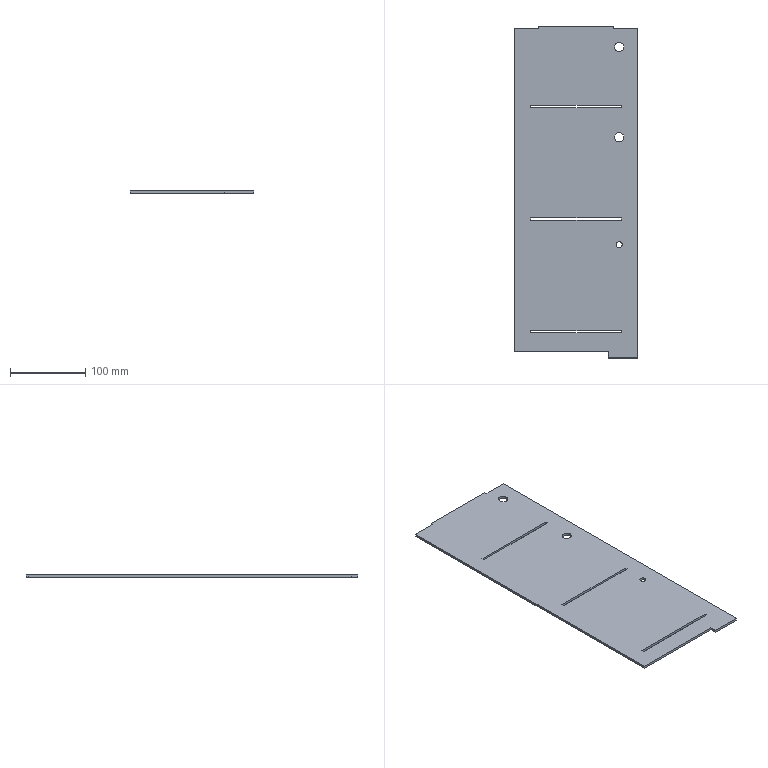Part | SolidWorks | features FlatPattern 1, SMBaseFlange 1, SheetMetal 1 | 1 solid | 30 faces | box 165 x 442 x 3.2 mm | volume 224791 mm3 | plane 24 | cylinder 6 | commonest cylinder face diameters 12.5 x4 8 x2
STEP:
#1=CARTESIAN_POINT('',(-21.25,194.5,3.2));
#2=VERTEX_POINT('',#1);
#3=CARTESIAN_POINT('',(-8.75,194.5,3.2));
#4=VERTEX_POINT('',#3);
#5=CARTESIAN_POINT('',(-15.,194.5,3.2));
#6=DIRECTION('',(0.,0.,1.));
#7=DIRECTION('',(1.,0.,0.));
#8=AXIS2_PLACEMENT_3D('',#5,#6,#7);
#9=CIRCLE('',#8,6.25);
#10=EDGE_CURVE('',#2,#4,#9,.T.);
#11=ORIENTED_EDGE('',*,*,#10,.T.);
#12=CARTESIAN_POINT('',(-8.75,194.5,0.));
#13=VERTEX_POINT('',#12);
#14=CARTESIAN_POINT('',(-8.75,194.5,3.2));
#15=DIRECTION('',(0.,0.,-1.));
#16=VECTOR('',#15,1000.);
#17=LINE('',#14,#16);
#18=EDGE_CURVE('',#4,#13,#17,.T.);
#19=ORIENTED_EDGE('',*,*,#18,.T.);
#20=CARTESIAN_POINT('',(-21.25,194.5,0.));
#21=VERTEX_POINT('',#20);
#22=CARTESIAN_POINT('',(-15.,194.5,0.));
#23=DIRECTION('',(0.,0.,1.));
#24=DIRECTION('',(1.,0.,0.));
#25=AXIS2_PLACEMENT_3D('',#22,#23,#24);
#26=CIRCLE('',#25,6.25);
#27=EDGE_CURVE('',#21,#13,#26,.T.);
#28=ORIENTED_EDGE('',*,*,#27,.F.);
#29=CARTESIAN_POINT('',(-21.25,194.5,3.2));
#30=DIRECTION('',(0.,0.,-1.));
#31=VECTOR('',#30,1000.);
#32=LINE('',#29,#31);
#33=EDGE_CURVE('',#2,#21,#32,.T.);
#34=ORIENTED_EDGE('',*,*,#33,.F.);
#35=EDGE_LOOP('',(#11,#19,#28,#34));
#36=FACE_OUTER_BOUND('',#35,.T.);
#37=CARTESIAN_POINT('',(-15.,194.5,3.2));
#38=DIRECTION('',(0.,0.,-1.));
#39=DIRECTION('',(-1.,0.,0.));
#40=AXIS2_PLACEMENT_3D('',#37,#38,#39);
#41=CYLINDRICAL_SURFACE('',#40,6.25);
#42=ADVANCED_FACE('',(#36),#41,.F.);
#43=CARTESIAN_POINT('',(-21.25,74.5,3.2));
#44=VERTEX_POINT('',#43);
#45=CARTESIAN_POINT('',(-8.75,74.5,3.2));
#46=VERTEX_POINT('',#45);
#47=CARTESIAN_POINT('',(-15.,74.5,3.2));
#48=DIRECTION('',(0.,0.,1.));
#49=DIRECTION('',(1.,0.,0.));
#50=AXIS2_PLACEMENT_3D('',#47,#48,#49);
#51=CIRCLE('',#50,6.25);
#52=EDGE_CURVE('',#44,#46,#51,.T.);
#53=ORIENTED_EDGE('',*,*,#52,.T.);
#54=CARTESIAN_POINT('',(-8.75,74.5,0.));
#55=VERTEX_POINT('',#54);
#56=CARTESIAN_POINT('',(-8.75,74.5,3.2));
#57=DIRECTION('',(0.,0.,-1.));
#58=VECTOR('',#57,1000.);
#59=LINE('',#56,#58);
#60=EDGE_CURVE('',#46,#55,#59,.T.);
#61=ORIENTED_EDGE('',*,*,#60,.T.);
#62=CARTESIAN_POINT('',(-21.25,74.5,0.));
#63=VERTEX_POINT('',#62);
#64=CARTESIAN_POINT('',(-15.,74.5,0.));
#65=DIRECTION('',(0.,0.,1.));
#66=DIRECTION('',(1.,0.,0.));
#67=AXIS2_PLACEMENT_3D('',#64,#65,#66);
#68=CIRCLE('',#67,6.25);
#69=EDGE_CURVE('',#63,#55,#68,.T.);
#70=ORIENTED_EDGE('',*,*,#69,.F.);
#71=CARTESIAN_POINT('',(-21.25,74.5,3.2));
#72=DIRECTION('',(0.,0.,-1.));
#73=VECTOR('',#72,1000.);
#74=LINE('',#71,#73);
#75=EDGE_CURVE('',#44,#63,#74,.T.);
#76=ORIENTED_EDGE('',*,*,#75,.F.);
#77=EDGE_LOOP('',(#53,#61,#70,#76));
#78=FACE_OUTER_BOUND('',#77,.T.);
#79=CARTESIAN_POINT('',(-15.,74.5,3.2));
#80=DIRECTION('',(0.,0.,-1.));
#81=DIRECTION('',(-1.,0.,0.));
#82=AXIS2_PLACEMENT_3D('',#79,#80,#81);
#83=CYLINDRICAL_SURFACE('',#82,6.25);
#84=ADVANCED_FACE('',(#78),#83,.F.);
#85=CARTESIAN_POINT('',(-19.,-68.5,3.2));
#86=VERTEX_POINT('',#85);
#87=CARTESIAN_POINT('',(-11.,-68.5,3.2));
#88=VERTEX_POINT('',#87);
#89=CARTESIAN_POINT('',(-15.,-68.5,3.2));
#90=DIRECTION('',(0.,0.,1.));
#91=DIRECTION('',(1.,0.,0.));
#92=AXIS2_PLACEMENT_3D('',#89,#90,#91);
#93=CIRCLE('',#92,4.);
#94=EDGE_CURVE('',#86,#88,#93,.T.);
#95=ORIENTED_EDGE('',*,*,#94,.T.);
#96=CARTESIAN_POINT('',(-11.,-68.5,0.));
#97=VERTEX_POINT('',#96);
#98=CARTESIAN_POINT('',(-11.,-68.5,3.2));
#99=DIRECTION('',(0.,0.,-1.));
#100=VECTOR('',#99,1000.);
#101=LINE('',#98,#100);
#102=EDGE_CURVE('',#88,#97,#101,.T.);
#103=ORIENTED_EDGE('',*,*,#102,.T.);
#104=CARTESIAN_POINT('',(-19.,-68.5,0.));
#105=VERTEX_POINT('',#104);
#106=CARTESIAN_POINT('',(-15.,-68.5,0.));
#107=DIRECTION('',(0.,0.,1.));
#108=DIRECTION('',(1.,0.,0.));
#109=AXIS2_PLACEMENT_3D('',#106,#107,#108);
#110=CIRCLE('',#109,4.);
#111=EDGE_CURVE('',#105,#97,#110,.T.);
#112=ORIENTED_EDGE('',*,*,#111,.F.);
#113=CARTESIAN_POINT('',(-19.,-68.5,3.2));
#114=DIRECTION('',(0.,0.,-1.));
#115=VECTOR('',#114,1000.);
#116=LINE('',#113,#115);
#117=EDGE_CURVE('',#86,#105,#116,.T.);
#118=ORIENTED_EDGE('',*,*,#117,.F.);
#119=EDGE_LOOP('',(#95,#103,#112,#118));
#120=FACE_OUTER_BOUND('',#119,.T.);
#121=CARTESIAN_POINT('',(-15.,-68.5,3.2));
#122=DIRECTION('',(0.,0.,-1.));
#123=DIRECTION('',(-1.,0.,0.));
#124=AXIS2_PLACEMENT_3D('',#121,#122,#123);
#125=CYLINDRICAL_SURFACE('',#124,4.);
#126=ADVANCED_FACE('',(#120),#125,.F.);
#127=ORIENTED_EDGE('',*,*,#52,.F.);
#128=CARTESIAN_POINT('',(-15.,74.5,3.2));
#129=DIRECTION('',(0.,0.,1.));
#130=DIRECTION('',(1.,0.,0.));
#131=AXIS2_PLACEMENT_3D('',#128,#129,#130);
#132=CIRCLE('',#131,6.25);
#133=EDGE_CURVE('',#46,#44,#132,.T.);
#134=ORIENTED_EDGE('',*,*,#133,.F.);
#135=EDGE_LOOP('',(#127,#134));
#136=FACE_BOUND('',#135,.T.);
#137=CARTESIAN_POINT('',(-122.5,219.5,3.2));
#138=VERTEX_POINT('',#137);
#139=CARTESIAN_POINT('',(-155.,219.5,3.2));
#140=VERTEX_POINT('',#139);
#141=CARTESIAN_POINT('',(-122.5,219.5,3.2));
#142=DIRECTION('',(-1.,0.,0.));
#143=VECTOR('',#142,1000.);
#144=LINE('',#141,#143);
#145=EDGE_CURVE('',#138,#140,#144,.T.);
#146=ORIENTED_EDGE('',*,*,#145,.T.);
#147=CARTESIAN_POINT('',(-155.,-211.2,3.2));
#148=VERTEX_POINT('',#147);
#149=CARTESIAN_POINT('',(-155.,219.5,3.2));
#150=DIRECTION('',(0.,-1.,0.));
#151=VECTOR('',#150,1000.);
#152=LINE('',#149,#151);
#153=EDGE_CURVE('',#140,#148,#152,.T.);
#154=ORIENTED_EDGE('',*,*,#153,.T.);
#155=CARTESIAN_POINT('',(-29.7,-211.2,3.2));
#156=VERTEX_POINT('',#155);
#157=CARTESIAN_POINT('',(-155.,-211.2,3.2));
#158=DIRECTION('',(1.,0.,0.));
#159=VECTOR('',#158,1000.);
#160=LINE('',#157,#159);
#161=EDGE_CURVE('',#148,#156,#160,.T.);
#162=ORIENTED_EDGE('',*,*,#161,.T.);
#163=CARTESIAN_POINT('',(-29.7,-219.5,3.2));
#164=VERTEX_POINT('',#163);
#165=CARTESIAN_POINT('',(-29.7,-211.2,3.2));
#166=DIRECTION('',(0.,-1.,0.));
#167=VECTOR('',#166,1000.);
#168=LINE('',#165,#167);
#169=EDGE_CURVE('',#156,#164,#168,.T.);
#170=ORIENTED_EDGE('',*,*,#169,.T.);
#171=CARTESIAN_POINT('',(10.,-219.5,3.2));
#172=VERTEX_POINT('',#171);
#173=CARTESIAN_POINT('',(-29.7,-219.5,3.2));
#174=DIRECTION('',(1.,0.,0.));
#175=VECTOR('',#174,1000.);
#176=LINE('',#173,#175);
#177=EDGE_CURVE('',#164,#172,#176,.T.);
#178=ORIENTED_EDGE('',*,*,#177,.T.);
#179=CARTESIAN_POINT('',(10.,219.5,3.2));
#180=VERTEX_POINT('',#179);
#181=CARTESIAN_POINT('',(10.,-219.5,3.2));
#182=DIRECTION('',(0.,1.,0.));
#183=VECTOR('',#182,1000.);
#184=LINE('',#181,#183);
#185=EDGE_CURVE('',#172,#180,#184,.T.);
#186=ORIENTED_EDGE('',*,*,#185,.T.);
#187=CARTESIAN_POINT('',(-22.5,219.5,3.2));
#188=VERTEX_POINT('',#187);
#189=CARTESIAN_POINT('',(10.,219.5,3.2));
#190=DIRECTION('',(-1.,0.,0.));
#191=VECTOR('',#190,1000.);
#192=LINE('',#189,#191);
#193=EDGE_CURVE('',#180,#188,#192,.T.);
#194=ORIENTED_EDGE('',*,*,#193,.T.);
#195=CARTESIAN_POINT('',(-22.5,222.5,3.2));
#196=VERTEX_POINT('',#195);
#197=CARTESIAN_POINT('',(-22.5,222.5,3.2));
#198=DIRECTION('',(0.,1.,0.));
#199=VECTOR('',#198,1000.);
#200=LINE('',#197,#199);
#201=EDGE_CURVE('',#188,#196,#200,.T.);
#202=ORIENTED_EDGE('',*,*,#201,.T.);
#203=CARTESIAN_POINT('',(-122.5,222.5,3.2));
#204=VERTEX_POINT('',#203);
#205=CARTESIAN_POINT('',(-122.5,222.5,3.2));
#206=DIRECTION('',(-1.,0.,0.));
#207=VECTOR('',#206,1000.);
#208=LINE('',#205,#207);
#209=EDGE_CURVE('',#196,#204,#208,.T.);
#210=ORIENTED_EDGE('',*,*,#209,.T.);
#211=CARTESIAN_POINT('',(-122.5,219.5,3.2));
#212=DIRECTION('',(0.,-1.,0.));
#213=VECTOR('',#212,1000.);
#214=LINE('',#211,#213);
#215=EDGE_CURVE('',#204,#138,#214,.T.);
#216=ORIENTED_EDGE('',*,*,#215,.T.);
#217=EDGE_LOOP('',(#146,#154,#162,#170,#178,#186,#194,#202,#210,#216));
#218=FACE_OUTER_BOUND('',#217,.T.);
#219=ORIENTED_EDGE('',*,*,#94,.F.);
#220=CARTESIAN_POINT('',(-15.,-68.5,3.2));
#221=DIRECTION('',(0.,0.,1.));
#222=DIRECTION('',(1.,0.,0.));
#223=AXIS2_PLACEMENT_3D('',#220,#221,#222);
#224=CIRCLE('',#223,4.);
#225=EDGE_CURVE('',#88,#86,#224,.T.);
#226=ORIENTED_EDGE('',*,*,#225,.F.);
#227=EDGE_LOOP('',(#219,#226));
#228=FACE_BOUND('',#227,.T.);
#229=ORIENTED_EDGE('',*,*,#10,.F.);
#230=CARTESIAN_POINT('',(-15.,194.5,3.2));
#231=DIRECTION('',(0.,0.,1.));
#232=DIRECTION('',(1.,0.,0.));
#233=AXIS2_PLACEMENT_3D('',#230,#231,#232);
#234=CIRCLE('',#233,6.25);
#235=EDGE_CURVE('',#4,#2,#234,.T.);
#236=ORIENTED_EDGE('',*,*,#235,.F.);
#237=EDGE_LOOP('',(#229,#236));
#238=FACE_BOUND('',#237,.T.);
#239=CARTESIAN_POINT('',(-132.5,-186.2,3.2));
#240=VERTEX_POINT('',#239);
#241=CARTESIAN_POINT('',(-12.5,-186.2,3.2));
#242=VERTEX_POINT('',#241);
#243=CARTESIAN_POINT('',(-132.5,-186.2,3.2));
#244=DIRECTION('',(1.,0.,0.));
#245=VECTOR('',#244,1000.);
#246=LINE('',#243,#245);
#247=EDGE_CURVE('',#240,#242,#246,.T.);
#248=ORIENTED_EDGE('',*,*,#247,.F.);
#249=CARTESIAN_POINT('',(-132.5,-183.,3.2));
#250=VERTEX_POINT('',#249);
#251=CARTESIAN_POINT('',(-132.5,-186.2,3.2));
#252=DIRECTION('',(0.,-1.,0.));
#253=VECTOR('',#252,1000.);
#254=LINE('',#251,#253);
#255=EDGE_CURVE('',#250,#240,#254,.T.);
#256=ORIENTED_EDGE('',*,*,#255,.F.);
#257=CARTESIAN_POINT('',(-12.5,-183.,3.2));
#258=VERTEX_POINT('',#257);
#259=CARTESIAN_POINT('',(-132.5,-183.,3.2));
#260=DIRECTION('',(-1.,0.,0.));
#261=VECTOR('',#260,1000.);
#262=LINE('',#259,#261);
#263=EDGE_CURVE('',#258,#250,#262,.T.);
#264=ORIENTED_EDGE('',*,*,#263,.F.);
#265=CARTESIAN_POINT('',(-12.5,-186.2,3.2));
#266=DIRECTION('',(0.,1.,0.));
#267=VECTOR('',#266,1000.);
#268=LINE('',#265,#267);
#269=EDGE_CURVE('',#242,#258,#268,.T.);
#270=ORIENTED_EDGE('',*,*,#269,.F.);
#271=EDGE_LOOP('',(#248,#256,#264,#270));
#272=FACE_BOUND('',#271,.T.);
#273=CARTESIAN_POINT('',(-132.5,-36.2,3.2));
#274=VERTEX_POINT('',#273);
#275=CARTESIAN_POINT('',(-12.5,-36.2,3.2));
#276=VERTEX_POINT('',#275);
#277=CARTESIAN_POINT('',(-132.5,-36.2,3.2));
#278=DIRECTION('',(1.,0.,0.));
#279=VECTOR('',#278,1000.);
#280=LINE('',#277,#279);
#281=EDGE_CURVE('',#274,#276,#280,.T.);
#282=ORIENTED_EDGE('',*,*,#281,.F.);
#283=CARTESIAN_POINT('',(-132.5,-33.,3.2));
#284=VERTEX_POINT('',#283);
#285=CARTESIAN_POINT('',(-132.5,-36.2,3.2));
#286=DIRECTION('',(0.,-1.,0.));
#287=VECTOR('',#286,1000.);
#288=LINE('',#285,#287);
#289=EDGE_CURVE('',#284,#274,#288,.T.);
#290=ORIENTED_EDGE('',*,*,#289,.F.);
#291=CARTESIAN_POINT('',(-12.5,-33.,3.2));
#292=VERTEX_POINT('',#291);
#293=CARTESIAN_POINT('',(-132.5,-33.,3.2));
#294=DIRECTION('',(-1.,0.,0.));
#295=VECTOR('',#294,1000.);
#296=LINE('',#293,#295);
#297=EDGE_CURVE('',#292,#284,#296,.T.);
#298=ORIENTED_EDGE('',*,*,#297,.F.);
#299=CARTESIAN_POINT('',(-12.5,-36.2,3.2));
#300=DIRECTION('',(0.,1.,0.));
#301=VECTOR('',#300,1000.);
#302=LINE('',#299,#301);
#303=EDGE_CURVE('',#276,#292,#302,.T.);
#304=ORIENTED_EDGE('',*,*,#303,.F.);
#305=EDGE_LOOP('',(#282,#290,#298,#304));
#306=FACE_BOUND('',#305,.T.);
#307=CARTESIAN_POINT('',(-132.5,113.8,3.2));
#308=VERTEX_POINT('',#307);
#309=CARTESIAN_POINT('',(-12.5,113.8,3.2));
#310=VERTEX_POINT('',#309);
#311=CARTESIAN_POINT('',(-132.5,113.8,3.2));
#312=DIRECTION('',(1.,0.,0.));
#313=VECTOR('',#312,1000.);
#314=LINE('',#311,#313);
#315=EDGE_CURVE('',#308,#310,#314,.T.);
#316=ORIENTED_EDGE('',*,*,#315,.F.);
#317=CARTESIAN_POINT('',(-132.5,117.,3.2));
#318=VERTEX_POINT('',#317);
#319=CARTESIAN_POINT('',(-132.5,113.8,3.2));
#320=DIRECTION('',(0.,-1.,0.));
#321=VECTOR('',#320,1000.);
#322=LINE('',#319,#321);
#323=EDGE_CURVE('',#318,#308,#322,.T.);
#324=ORIENTED_EDGE('',*,*,#323,.F.);
#325=CARTESIAN_POINT('',(-12.5,117.,3.2));
#326=VERTEX_POINT('',#325);
#327=CARTESIAN_POINT('',(-132.5,117.,3.2));
#328=DIRECTION('',(-1.,0.,0.));
#329=VECTOR('',#328,1000.);
#330=LINE('',#327,#329);
#331=EDGE_CURVE('',#326,#318,#330,.T.);
#332=ORIENTED_EDGE('',*,*,#331,.F.);
#333=CARTESIAN_POINT('',(-12.5,113.8,3.2));
#334=DIRECTION('',(0.,1.,0.));
#335=VECTOR('',#334,1000.);
#336=LINE('',#333,#335);
#337=EDGE_CURVE('',#310,#326,#336,.T.);
#338=ORIENTED_EDGE('',*,*,#337,.F.);
#339=EDGE_LOOP('',(#316,#324,#332,#338));
#340=FACE_BOUND('',#339,.T.);
#341=CARTESIAN_POINT('',(0.,0.,3.2));
#342=DIRECTION('',(0.,0.,1.));
#343=DIRECTION('',(1.,0.,0.));
#344=AXIS2_PLACEMENT_3D('',#341,#342,#343);
#345=PLANE('',#344);
#346=ADVANCED_FACE('',(#136,#218,#228,#238,#272,#306,#340),#345,.T.);
#347=CARTESIAN_POINT('',(-132.5,-33.,0.));
#348=VERTEX_POINT('',#347);
#349=CARTESIAN_POINT('',(-132.5,-36.2,0.));
#350=VERTEX_POINT('',#349);
#351=CARTESIAN_POINT('',(-132.5,-36.2,0.));
#352=DIRECTION('',(0.,-1.,0.));
#353=VECTOR('',#352,1000.);
#354=LINE('',#351,#353);
#355=EDGE_CURVE('',#348,#350,#354,.T.);
#356=ORIENTED_EDGE('',*,*,#355,.T.);
#357=CARTESIAN_POINT('',(-12.5,-36.2,0.));
#358=VERTEX_POINT('',#357);
#359=CARTESIAN_POINT('',(-132.5,-36.2,0.));
#360=DIRECTION('',(1.,0.,0.));
#361=VECTOR('',#360,1000.);
#362=LINE('',#359,#361);
#363=EDGE_CURVE('',#350,#358,#362,.T.);
#364=ORIENTED_EDGE('',*,*,#363,.T.);
#365=CARTESIAN_POINT('',(-12.5,-33.,0.));
#366=VERTEX_POINT('',#365);
#367=CARTESIAN_POINT('',(-12.5,-36.2,0.));
#368=DIRECTION('',(0.,1.,0.));
#369=VECTOR('',#368,1000.);
#370=LINE('',#367,#369);
#371=EDGE_CURVE('',#358,#366,#370,.T.);
#372=ORIENTED_EDGE('',*,*,#371,.T.);
#373=CARTESIAN_POINT('',(-132.5,-33.,0.));
#374=DIRECTION('',(-1.,0.,0.));
#375=VECTOR('',#374,1000.);
#376=LINE('',#373,#375);
#377=EDGE_CURVE('',#366,#348,#376,.T.);
#378=ORIENTED_EDGE('',*,*,#377,.T.);
#379=EDGE_LOOP('',(#356,#364,#372,#378));
#380=FACE_BOUND('',#379,.T.);
#381=ORIENTED_EDGE('',*,*,#27,.T.);
#382=CARTESIAN_POINT('',(-15.,194.5,0.));
#383=DIRECTION('',(0.,0.,1.));
#384=DIRECTION('',(1.,0.,0.));
#385=AXIS2_PLACEMENT_3D('',#382,#383,#384);
#386=CIRCLE('',#385,6.25);
#387=EDGE_CURVE('',#13,#21,#386,.T.);
#388=ORIENTED_EDGE('',*,*,#387,.T.);
#389=EDGE_LOOP('',(#381,#388));
#390=FACE_BOUND('',#389,.T.);
#391=ORIENTED_EDGE('',*,*,#69,.T.);
#392=CARTESIAN_POINT('',(-15.,74.5,0.));
#393=DIRECTION('',(0.,0.,1.));
#394=DIRECTION('',(1.,0.,0.));
#395=AXIS2_PLACEMENT_3D('',#392,#393,#394);
#396=CIRCLE('',#395,6.25);
#397=EDGE_CURVE('',#55,#63,#396,.T.);
#398=ORIENTED_EDGE('',*,*,#397,.T.);
#399=EDGE_LOOP('',(#391,#398));
#400=FACE_BOUND('',#399,.T.);
#401=ORIENTED_EDGE('',*,*,#111,.T.);
#402=CARTESIAN_POINT('',(-15.,-68.5,0.));
#403=DIRECTION('',(0.,0.,1.));
#404=DIRECTION('',(1.,0.,0.));
#405=AXIS2_PLACEMENT_3D('',#402,#403,#404);
#406=CIRCLE('',#405,4.);
#407=EDGE_CURVE('',#97,#105,#406,.T.);
#408=ORIENTED_EDGE('',*,*,#407,.T.);
#409=EDGE_LOOP('',(#401,#408));
#410=FACE_BOUND('',#409,.T.);
#411=CARTESIAN_POINT('',(-122.5,219.5,0.));
#412=VERTEX_POINT('',#411);
#413=CARTESIAN_POINT('',(-155.,219.5,0.));
#414=VERTEX_POINT('',#413);
#415=CARTESIAN_POINT('',(-122.5,219.5,0.));
#416=DIRECTION('',(-1.,0.,0.));
#417=VECTOR('',#416,1000.);
#418=LINE('',#415,#417);
#419=EDGE_CURVE('',#412,#414,#418,.T.);
#420=ORIENTED_EDGE('',*,*,#419,.F.);
#421=CARTESIAN_POINT('',(-122.5,222.5,0.));
#422=VERTEX_POINT('',#421);
#423=CARTESIAN_POINT('',(-122.5,219.5,0.));
#424=DIRECTION('',(0.,-1.,0.));
#425=VECTOR('',#424,1000.);
#426=LINE('',#423,#425);
#427=EDGE_CURVE('',#422,#412,#426,.T.);
#428=ORIENTED_EDGE('',*,*,#427,.F.);
#429=CARTESIAN_POINT('',(-22.5,222.5,0.));
#430=VERTEX_POINT('',#429);
#431=CARTESIAN_POINT('',(-122.5,222.5,0.));
#432=DIRECTION('',(-1.,0.,0.));
#433=VECTOR('',#432,1000.);
#434=LINE('',#431,#433);
#435=EDGE_CURVE('',#430,#422,#434,.T.);
#436=ORIENTED_EDGE('',*,*,#435,.F.);
#437=CARTESIAN_POINT('',(-22.5,219.5,0.));
#438=VERTEX_POINT('',#437);
#439=CARTESIAN_POINT('',(-22.5,222.5,0.));
#440=DIRECTION('',(0.,1.,0.));
#441=VECTOR('',#440,1000.);
#442=LINE('',#439,#441);
#443=EDGE_CURVE('',#438,#430,#442,.T.);
#444=ORIENTED_EDGE('',*,*,#443,.F.);
#445=CARTESIAN_POINT('',(10.,219.5,0.));
#446=VERTEX_POINT('',#445);
#447=CARTESIAN_POINT('',(10.,219.5,0.));
#448=DIRECTION('',(-1.,0.,0.));
#449=VECTOR('',#448,1000.);
#450=LINE('',#447,#449);
#451=EDGE_CURVE('',#446,#438,#450,.T.);
#452=ORIENTED_EDGE('',*,*,#451,.F.);
#453=CARTESIAN_POINT('',(10.,-219.5,0.));
#454=VERTEX_POINT('',#453);
#455=CARTESIAN_POINT('',(10.,-219.5,0.));
#456=DIRECTION('',(0.,1.,0.));
#457=VECTOR('',#456,1000.);
#458=LINE('',#455,#457);
#459=EDGE_CURVE('',#454,#446,#458,.T.);
#460=ORIENTED_EDGE('',*,*,#459,.F.);
#461=CARTESIAN_POINT('',(-29.7,-219.5,0.));
#462=VERTEX_POINT('',#461);
#463=CARTESIAN_POINT('',(-29.7,-219.5,0.));
#464=DIRECTION('',(1.,0.,0.));
#465=VECTOR('',#464,1000.);
#466=LINE('',#463,#465);
#467=EDGE_CURVE('',#462,#454,#466,.T.);
#468=ORIENTED_EDGE('',*,*,#467,.F.);
#469=CARTESIAN_POINT('',(-29.7,-211.2,0.));
#470=VERTEX_POINT('',#469);
#471=CARTESIAN_POINT('',(-29.7,-211.2,0.));
#472=DIRECTION('',(0.,-1.,0.));
#473=VECTOR('',#472,1000.);
#474=LINE('',#471,#473);
#475=EDGE_CURVE('',#470,#462,#474,.T.);
#476=ORIENTED_EDGE('',*,*,#475,.F.);
#477=CARTESIAN_POINT('',(-155.,-211.2,0.));
#478=VERTEX_POINT('',#477);
#479=CARTESIAN_POINT('',(-155.,-211.2,0.));
#480=DIRECTION('',(1.,0.,0.));
#481=VECTOR('',#480,1000.);
#482=LINE('',#479,#481);
#483=EDGE_CURVE('',#478,#470,#482,.T.);
#484=ORIENTED_EDGE('',*,*,#483,.F.);
#485=CARTESIAN_POINT('',(-155.,219.5,0.));
#486=DIRECTION('',(0.,-1.,0.));
#487=VECTOR('',#486,1000.);
#488=LINE('',#485,#487);
#489=EDGE_CURVE('',#414,#478,#488,.T.);
#490=ORIENTED_EDGE('',*,*,#489,.F.);
#491=EDGE_LOOP('',(#420,#428,#436,#444,#452,#460,#468,#476,#484,#490));
#492=FACE_OUTER_BOUND('',#491,.T.);
#493=CARTESIAN_POINT('',(-132.5,-183.,0.));
#494=VERTEX_POINT('',#493);
#495=CARTESIAN_POINT('',(-132.5,-186.2,0.));
#496=VERTEX_POINT('',#495);
#497=CARTESIAN_POINT('',(-132.5,-186.2,0.));
#498=DIRECTION('',(0.,-1.,0.));
#499=VECTOR('',#498,1000.);
#500=LINE('',#497,#499);
#501=EDGE_CURVE('',#494,#496,#500,.T.);
#502=ORIENTED_EDGE('',*,*,#501,.T.);
#503=CARTESIAN_POINT('',(-12.5,-186.2,0.));
#504=VERTEX_POINT('',#503);
#505=CARTESIAN_POINT('',(-132.5,-186.2,0.));
#506=DIRECTION('',(1.,0.,0.));
#507=VECTOR('',#506,1000.);
#508=LINE('',#505,#507);
#509=EDGE_CURVE('',#496,#504,#508,.T.);
#510=ORIENTED_EDGE('',*,*,#509,.T.);
#511=CARTESIAN_POINT('',(-12.5,-183.,0.));
#512=VERTEX_POINT('',#511);
#513=CARTESIAN_POINT('',(-12.5,-186.2,0.));
#514=DIRECTION('',(0.,1.,0.));
#515=VECTOR('',#514,1000.);
#516=LINE('',#513,#515);
#517=EDGE_CURVE('',#504,#512,#516,.T.);
#518=ORIENTED_EDGE('',*,*,#517,.T.);
#519=CARTESIAN_POINT('',(-132.5,-183.,0.));
#520=DIRECTION('',(-1.,0.,0.));
#521=VECTOR('',#520,1000.);
#522=LINE('',#519,#521);
#523=EDGE_CURVE('',#512,#494,#522,.T.);
#524=ORIENTED_EDGE('',*,*,#523,.T.);
#525=EDGE_LOOP('',(#502,#510,#518,#524));
#526=FACE_BOUND('',#525,.T.);
#527=CARTESIAN_POINT('',(-132.5,117.,0.));
#528=VERTEX_POINT('',#527);
#529=CARTESIAN_POINT('',(-132.5,113.8,0.));
#530=VERTEX_POINT('',#529);
#531=CARTESIAN_POINT('',(-132.5,113.8,0.));
#532=DIRECTION('',(0.,-1.,0.));
#533=VECTOR('',#532,1000.);
#534=LINE('',#531,#533);
#535=EDGE_CURVE('',#528,#530,#534,.T.);
#536=ORIENTED_EDGE('',*,*,#535,.T.);
#537=CARTESIAN_POINT('',(-12.5,113.8,0.));
#538=VERTEX_POINT('',#537);
#539=CARTESIAN_POINT('',(-132.5,113.8,0.));
#540=DIRECTION('',(1.,0.,0.));
#541=VECTOR('',#540,1000.);
#542=LINE('',#539,#541);
#543=EDGE_CURVE('',#530,#538,#542,.T.);
#544=ORIENTED_EDGE('',*,*,#543,.T.);
#545=CARTESIAN_POINT('',(-12.5,117.,0.));
#546=VERTEX_POINT('',#545);
#547=CARTESIAN_POINT('',(-12.5,113.8,0.));
#548=DIRECTION('',(0.,1.,0.));
#549=VECTOR('',#548,1000.);
#550=LINE('',#547,#549);
#551=EDGE_CURVE('',#538,#546,#550,.T.);
#552=ORIENTED_EDGE('',*,*,#551,.T.);
#553=CARTESIAN_POINT('',(-132.5,117.,0.));
#554=DIRECTION('',(-1.,0.,0.));
#555=VECTOR('',#554,1000.);
#556=LINE('',#553,#555);
#557=EDGE_CURVE('',#546,#528,#556,.T.);
#558=ORIENTED_EDGE('',*,*,#557,.T.);
#559=EDGE_LOOP('',(#536,#544,#552,#558));
#560=FACE_BOUND('',#559,.T.);
#561=CARTESIAN_POINT('',(0.,0.,0.));
#562=DIRECTION('',(0.,0.,1.));
#563=DIRECTION('',(1.,0.,0.));
#564=AXIS2_PLACEMENT_3D('',#561,#562,#563);
#565=PLANE('',#564);
#566=ADVANCED_FACE('',(#380,#390,#400,#410,#492,#526,#560),#565,.F.);
#567=ORIENTED_EDGE('',*,*,#419,.T.);
#568=CARTESIAN_POINT('',(-155.,219.5,3.2));
#569=DIRECTION('',(0.,0.,-1.));
#570=VECTOR('',#569,1000.);
#571=LINE('',#568,#570);
#572=EDGE_CURVE('',#140,#414,#571,.T.);
#573=ORIENTED_EDGE('',*,*,#572,.F.);
#574=ORIENTED_EDGE('',*,*,#145,.F.);
#575=CARTESIAN_POINT('',(-122.5,219.5,3.2));
#576=DIRECTION('',(0.,0.,-1.));
#577=VECTOR('',#576,1000.);
#578=LINE('',#575,#577);
#579=EDGE_CURVE('',#138,#412,#578,.T.);
#580=ORIENTED_EDGE('',*,*,#579,.T.);
#581=EDGE_LOOP('',(#567,#573,#574,#580));
#582=FACE_OUTER_BOUND('',#581,.T.);
#583=CARTESIAN_POINT('',(-122.5,219.5,3.2));
#584=DIRECTION('',(0.,-1.,0.));
#585=DIRECTION('',(0.,0.,-1.));
#586=AXIS2_PLACEMENT_3D('',#583,#584,#585);
#587=PLANE('',#586);
#588=ADVANCED_FACE('',(#582),#587,.F.);
#589=ORIENTED_EDGE('',*,*,#489,.T.);
#590=CARTESIAN_POINT('',(-155.,-211.2,3.2));
#591=DIRECTION('',(0.,0.,-1.));
#592=VECTOR('',#591,1000.);
#593=LINE('',#590,#592);
#594=EDGE_CURVE('',#148,#478,#593,.T.);
#595=ORIENTED_EDGE('',*,*,#594,.F.);
#596=ORIENTED_EDGE('',*,*,#153,.F.);
#597=ORIENTED_EDGE('',*,*,#572,.T.);
#598=EDGE_LOOP('',(#589,#595,#596,#597));
#599=FACE_OUTER_BOUND('',#598,.T.);
#600=CARTESIAN_POINT('',(-155.,219.5,3.2));
#601=DIRECTION('',(1.,0.,0.));
#602=DIRECTION('',(0.,1.,0.));
#603=AXIS2_PLACEMENT_3D('',#600,#601,#602);
#604=PLANE('',#603);
#605=ADVANCED_FACE('',(#599),#604,.F.);
#606=ORIENTED_EDGE('',*,*,#483,.T.);
#607=CARTESIAN_POINT('',(-29.7,-211.2,3.2));
#608=DIRECTION('',(0.,0.,-1.));
#609=VECTOR('',#608,1000.);
#610=LINE('',#607,#609);
#611=EDGE_CURVE('',#156,#470,#610,.T.);
#612=ORIENTED_EDGE('',*,*,#611,.F.);
#613=ORIENTED_EDGE('',*,*,#161,.F.);
#614=ORIENTED_EDGE('',*,*,#594,.T.);
#615=EDGE_LOOP('',(#606,#612,#613,#614));
#616=FACE_OUTER_BOUND('',#615,.T.);
#617=CARTESIAN_POINT('',(-155.,-211.2,3.2));
#618=DIRECTION('',(0.,1.,0.));
#619=DIRECTION('',(-1.,0.,0.));
#620=AXIS2_PLACEMENT_3D('',#617,#618,#619);
#621=PLANE('',#620);
#622=ADVANCED_FACE('',(#616),#621,.F.);
#623=ORIENTED_EDGE('',*,*,#475,.T.);
#624=CARTESIAN_POINT('',(-29.7,-219.5,3.2));
#625=DIRECTION('',(0.,0.,-1.));
#626=VECTOR('',#625,1000.);
#627=LINE('',#624,#626);
#628=EDGE_CURVE('',#164,#462,#627,.T.);
#629=ORIENTED_EDGE('',*,*,#628,.F.);
#630=ORIENTED_EDGE('',*,*,#169,.F.);
#631=ORIENTED_EDGE('',*,*,#611,.T.);
#632=EDGE_LOOP('',(#623,#629,#630,#631));
#633=FACE_OUTER_BOUND('',#632,.T.);
#634=CARTESIAN_POINT('',(-29.7,-211.2,3.2));
#635=DIRECTION('',(1.,0.,0.));
#636=DIRECTION('',(0.,0.,-1.));
#637=AXIS2_PLACEMENT_3D('',#634,#635,#636);
#638=PLANE('',#637);
#639=ADVANCED_FACE('',(#633),#638,.F.);
#640=ORIENTED_EDGE('',*,*,#467,.T.);
#641=CARTESIAN_POINT('',(10.,-219.5,3.2));
#642=DIRECTION('',(0.,0.,-1.));
#643=VECTOR('',#642,1000.);
#644=LINE('',#641,#643);
#645=EDGE_CURVE('',#172,#454,#644,.T.);
#646=ORIENTED_EDGE('',*,*,#645,.F.);
#647=ORIENTED_EDGE('',*,*,#177,.F.);
#648=ORIENTED_EDGE('',*,*,#628,.T.);
#649=EDGE_LOOP('',(#640,#646,#647,#648));
#650=FACE_OUTER_BOUND('',#649,.T.);
#651=CARTESIAN_POINT('',(-29.7,-219.5,3.2));
#652=DIRECTION('',(0.,1.,0.));
#653=DIRECTION('',(0.,0.,1.));
#654=AXIS2_PLACEMENT_3D('',#651,#652,#653);
#655=PLANE('',#654);
#656=ADVANCED_FACE('',(#650),#655,.F.);
#657=ORIENTED_EDGE('',*,*,#459,.T.);
#658=CARTESIAN_POINT('',(10.,219.5,3.2));
#659=DIRECTION('',(0.,0.,-1.));
#660=VECTOR('',#659,1000.);
#661=LINE('',#658,#660);
#662=EDGE_CURVE('',#180,#446,#661,.T.);
#663=ORIENTED_EDGE('',*,*,#662,.F.);
#664=ORIENTED_EDGE('',*,*,#185,.F.);
#665=ORIENTED_EDGE('',*,*,#645,.T.);
#666=EDGE_LOOP('',(#657,#663,#664,#665));
#667=FACE_OUTER_BOUND('',#666,.T.);
#668=CARTESIAN_POINT('',(10.,-219.5,3.2));
#669=DIRECTION('',(-1.,0.,0.));
#670=DIRECTION('',(0.,0.,1.));
#671=AXIS2_PLACEMENT_3D('',#668,#669,#670);
#672=PLANE('',#671);
#673=ADVANCED_FACE('',(#667),#672,.F.);
#674=ORIENTED_EDGE('',*,*,#451,.T.);
#675=CARTESIAN_POINT('',(-22.5,219.5,3.2));
#676=DIRECTION('',(0.,0.,-1.));
#677=VECTOR('',#676,1000.);
#678=LINE('',#675,#677);
#679=EDGE_CURVE('',#188,#438,#678,.T.);
#680=ORIENTED_EDGE('',*,*,#679,.F.);
#681=ORIENTED_EDGE('',*,*,#193,.F.);
#682=ORIENTED_EDGE('',*,*,#662,.T.);
#683=EDGE_LOOP('',(#674,#680,#681,#682));
#684=FACE_OUTER_BOUND('',#683,.T.);
#685=CARTESIAN_POINT('',(10.,219.5,3.2));
#686=DIRECTION('',(0.,-1.,0.));
#687=DIRECTION('',(0.,0.,-1.));
#688=AXIS2_PLACEMENT_3D('',#685,#686,#687);
#689=PLANE('',#688);
#690=ADVANCED_FACE('',(#684),#689,.F.);
#691=ORIENTED_EDGE('',*,*,#443,.T.);
#692=CARTESIAN_POINT('',(-22.5,222.5,3.2));
#693=DIRECTION('',(0.,0.,-1.));
#694=VECTOR('',#693,1000.);
#695=LINE('',#692,#694);
#696=EDGE_CURVE('',#196,#430,#695,.T.);
#697=ORIENTED_EDGE('',*,*,#696,.F.);
#698=ORIENTED_EDGE('',*,*,#201,.F.);
#699=ORIENTED_EDGE('',*,*,#679,.T.);
#700=EDGE_LOOP('',(#691,#697,#698,#699));
#701=FACE_OUTER_BOUND('',#700,.T.);
#702=CARTESIAN_POINT('',(-22.5,222.5,3.2));
#703=DIRECTION('',(-1.,0.,0.));
#704=DIRECTION('',(0.,0.,1.));
#705=AXIS2_PLACEMENT_3D('',#702,#703,#704);
#706=PLANE('',#705);
#707=ADVANCED_FACE('',(#701),#706,.F.);
#708=ORIENTED_EDGE('',*,*,#435,.T.);
#709=CARTESIAN_POINT('',(-122.5,222.5,3.2));
#710=DIRECTION('',(0.,0.,-1.));
#711=VECTOR('',#710,1000.);
#712=LINE('',#709,#711);
#713=EDGE_CURVE('',#204,#422,#712,.T.);
#714=ORIENTED_EDGE('',*,*,#713,.F.);
#715=ORIENTED_EDGE('',*,*,#209,.F.);
#716=ORIENTED_EDGE('',*,*,#696,.T.);
#717=EDGE_LOOP('',(#708,#714,#715,#716));
#718=FACE_OUTER_BOUND('',#717,.T.);
#719=CARTESIAN_POINT('',(-122.5,222.5,3.2));
#720=DIRECTION('',(0.,-1.,0.));
#721=DIRECTION('',(0.,0.,-1.));
#722=AXIS2_PLACEMENT_3D('',#719,#720,#721);
#723=PLANE('',#722);
#724=ADVANCED_FACE('',(#718),#723,.F.);
#725=ORIENTED_EDGE('',*,*,#427,.T.);
#726=ORIENTED_EDGE('',*,*,#579,.F.);
#727=ORIENTED_EDGE('',*,*,#215,.F.);
#728=ORIENTED_EDGE('',*,*,#713,.T.);
#729=EDGE_LOOP('',(#725,#726,#727,#728));
#730=FACE_OUTER_BOUND('',#729,.T.);
#731=CARTESIAN_POINT('',(-122.5,219.5,3.2));
#732=DIRECTION('',(1.,0.,0.));
#733=DIRECTION('',(0.,0.,-1.));
#734=AXIS2_PLACEMENT_3D('',#731,#732,#733);
#735=PLANE('',#734);
#736=ADVANCED_FACE('',(#730),#735,.F.);
#737=ORIENTED_EDGE('',*,*,#102,.F.);
#738=ORIENTED_EDGE('',*,*,#225,.T.);
#739=ORIENTED_EDGE('',*,*,#117,.T.);
#740=ORIENTED_EDGE('',*,*,#407,.F.);
#741=EDGE_LOOP('',(#737,#738,#739,#740));
#742=FACE_OUTER_BOUND('',#741,.T.);
#743=CARTESIAN_POINT('',(-15.,-68.5,3.2));
#744=DIRECTION('',(0.,0.,-1.));
#745=DIRECTION('',(-1.,0.,0.));
#746=AXIS2_PLACEMENT_3D('',#743,#744,#745);
#747=CYLINDRICAL_SURFACE('',#746,4.);
#748=ADVANCED_FACE('',(#742),#747,.F.);
#749=ORIENTED_EDGE('',*,*,#60,.F.);
#750=ORIENTED_EDGE('',*,*,#133,.T.);
#751=ORIENTED_EDGE('',*,*,#75,.T.);
#752=ORIENTED_EDGE('',*,*,#397,.F.);
#753=EDGE_LOOP('',(#749,#750,#751,#752));
#754=FACE_OUTER_BOUND('',#753,.T.);
#755=CARTESIAN_POINT('',(-15.,74.5,3.2));
#756=DIRECTION('',(0.,0.,-1.));
#757=DIRECTION('',(-1.,0.,0.));
#758=AXIS2_PLACEMENT_3D('',#755,#756,#757);
#759=CYLINDRICAL_SURFACE('',#758,6.25);
#760=ADVANCED_FACE('',(#754),#759,.F.);
#761=ORIENTED_EDGE('',*,*,#18,.F.);
#762=ORIENTED_EDGE('',*,*,#235,.T.);
#763=ORIENTED_EDGE('',*,*,#33,.T.);
#764=ORIENTED_EDGE('',*,*,#387,.F.);
#765=EDGE_LOOP('',(#761,#762,#763,#764));
#766=FACE_OUTER_BOUND('',#765,.T.);
#767=CARTESIAN_POINT('',(-15.,194.5,3.2));
#768=DIRECTION('',(0.,0.,-1.));
#769=DIRECTION('',(-1.,0.,0.));
#770=AXIS2_PLACEMENT_3D('',#767,#768,#769);
#771=CYLINDRICAL_SURFACE('',#770,6.25);
#772=ADVANCED_FACE('',(#766),#771,.F.);
#773=ORIENTED_EDGE('',*,*,#501,.F.);
#774=CARTESIAN_POINT('',(-132.5,-183.,3.2));
#775=DIRECTION('',(0.,0.,-1.));
#776=VECTOR('',#775,1000.);
#777=LINE('',#774,#776);
#778=EDGE_CURVE('',#250,#494,#777,.T.);
#779=ORIENTED_EDGE('',*,*,#778,.F.);
#780=ORIENTED_EDGE('',*,*,#255,.T.);
#781=CARTESIAN_POINT('',(-132.5,-186.2,3.2));
#782=DIRECTION('',(0.,0.,-1.));
#783=VECTOR('',#782,1000.);
#784=LINE('',#781,#783);
#785=EDGE_CURVE('',#240,#496,#784,.T.);
#786=ORIENTED_EDGE('',*,*,#785,.T.);
#787=EDGE_LOOP('',(#773,#779,#780,#786));
#788=FACE_OUTER_BOUND('',#787,.T.);
#789=CARTESIAN_POINT('',(-132.5,-186.2,3.2));
#790=DIRECTION('',(1.,0.,0.));
#791=DIRECTION('',(0.,0.,-1.));
#792=AXIS2_PLACEMENT_3D('',#789,#790,#791);
#793=PLANE('',#792);
#794=ADVANCED_FACE('',(#788),#793,.T.);
#795=ORIENTED_EDGE('',*,*,#509,.F.);
#796=ORIENTED_EDGE('',*,*,#785,.F.);
#797=ORIENTED_EDGE('',*,*,#247,.T.);
#798=CARTESIAN_POINT('',(-12.5,-186.2,3.2));
#799=DIRECTION('',(0.,0.,-1.));
#800=VECTOR('',#799,1000.);
#801=LINE('',#798,#800);
#802=EDGE_CURVE('',#242,#504,#801,.T.);
#803=ORIENTED_EDGE('',*,*,#802,.T.);
#804=EDGE_LOOP('',(#795,#796,#797,#803));
#805=FACE_OUTER_BOUND('',#804,.T.);
#806=CARTESIAN_POINT('',(-132.5,-186.2,3.2));
#807=DIRECTION('',(0.,1.,0.));
#808=DIRECTION('',(0.,0.,1.));
#809=AXIS2_PLACEMENT_3D('',#806,#807,#808);
#810=PLANE('',#809);
#811=ADVANCED_FACE('',(#805),#810,.T.);
#812=ORIENTED_EDGE('',*,*,#517,.F.);
#813=ORIENTED_EDGE('',*,*,#802,.F.);
#814=ORIENTED_EDGE('',*,*,#269,.T.);
#815=CARTESIAN_POINT('',(-12.5,-183.,3.2));
#816=DIRECTION('',(0.,0.,-1.));
#817=VECTOR('',#816,1000.);
#818=LINE('',#815,#817);
#819=EDGE_CURVE('',#258,#512,#818,.T.);
#820=ORIENTED_EDGE('',*,*,#819,.T.);
#821=EDGE_LOOP('',(#812,#813,#814,#820));
#822=FACE_OUTER_BOUND('',#821,.T.);
#823=CARTESIAN_POINT('',(-12.5,-186.2,3.2));
#824=DIRECTION('',(-1.,0.,0.));
#825=DIRECTION('',(0.,0.,1.));
#826=AXIS2_PLACEMENT_3D('',#823,#824,#825);
#827=PLANE('',#826);
#828=ADVANCED_FACE('',(#822),#827,.T.);
#829=ORIENTED_EDGE('',*,*,#523,.F.);
#830=ORIENTED_EDGE('',*,*,#819,.F.);
#831=ORIENTED_EDGE('',*,*,#263,.T.);
#832=ORIENTED_EDGE('',*,*,#778,.T.);
#833=EDGE_LOOP('',(#829,#830,#831,#832));
#834=FACE_OUTER_BOUND('',#833,.T.);
#835=CARTESIAN_POINT('',(-132.5,-183.,3.2));
#836=DIRECTION('',(0.,-1.,0.));
#837=DIRECTION('',(0.,0.,-1.));
#838=AXIS2_PLACEMENT_3D('',#835,#836,#837);
#839=PLANE('',#838);
#840=ADVANCED_FACE('',(#834),#839,.T.);
#841=ORIENTED_EDGE('',*,*,#355,.F.);
#842=CARTESIAN_POINT('',(-132.5,-33.,3.2));
#843=DIRECTION('',(0.,0.,-1.));
#844=VECTOR('',#843,1000.);
#845=LINE('',#842,#844);
#846=EDGE_CURVE('',#284,#348,#845,.T.);
#847=ORIENTED_EDGE('',*,*,#846,.F.);
#848=ORIENTED_EDGE('',*,*,#289,.T.);
#849=CARTESIAN_POINT('',(-132.5,-36.2,3.2));
#850=DIRECTION('',(0.,0.,-1.));
#851=VECTOR('',#850,1000.);
#852=LINE('',#849,#851);
#853=EDGE_CURVE('',#274,#350,#852,.T.);
#854=ORIENTED_EDGE('',*,*,#853,.T.);
#855=EDGE_LOOP('',(#841,#847,#848,#854));
#856=FACE_OUTER_BOUND('',#855,.T.);
#857=CARTESIAN_POINT('',(-132.5,-36.2,3.2));
#858=DIRECTION('',(1.,0.,0.));
#859=DIRECTION('',(0.,0.,-1.));
#860=AXIS2_PLACEMENT_3D('',#857,#858,#859);
#861=PLANE('',#860);
#862=ADVANCED_FACE('',(#856),#861,.T.);
#863=ORIENTED_EDGE('',*,*,#363,.F.);
#864=ORIENTED_EDGE('',*,*,#853,.F.);
#865=ORIENTED_EDGE('',*,*,#281,.T.);
#866=CARTESIAN_POINT('',(-12.5,-36.2,3.2));
#867=DIRECTION('',(0.,0.,-1.));
#868=VECTOR('',#867,1000.);
#869=LINE('',#866,#868);
#870=EDGE_CURVE('',#276,#358,#869,.T.);
#871=ORIENTED_EDGE('',*,*,#870,.T.);
#872=EDGE_LOOP('',(#863,#864,#865,#871));
#873=FACE_OUTER_BOUND('',#872,.T.);
#874=CARTESIAN_POINT('',(-132.5,-36.2,3.2));
#875=DIRECTION('',(0.,1.,0.));
#876=DIRECTION('',(0.,0.,1.));
#877=AXIS2_PLACEMENT_3D('',#874,#875,#876);
#878=PLANE('',#877);
#879=ADVANCED_FACE('',(#873),#878,.T.);
#880=ORIENTED_EDGE('',*,*,#371,.F.);
#881=ORIENTED_EDGE('',*,*,#870,.F.);
#882=ORIENTED_EDGE('',*,*,#303,.T.);
#883=CARTESIAN_POINT('',(-12.5,-33.,3.2));
#884=DIRECTION('',(0.,0.,-1.));
#885=VECTOR('',#884,1000.);
#886=LINE('',#883,#885);
#887=EDGE_CURVE('',#292,#366,#886,.T.);
#888=ORIENTED_EDGE('',*,*,#887,.T.);
#889=EDGE_LOOP('',(#880,#881,#882,#888));
#890=FACE_OUTER_BOUND('',#889,.T.);
#891=CARTESIAN_POINT('',(-12.5,-36.2,3.2));
#892=DIRECTION('',(-1.,0.,0.));
#893=DIRECTION('',(0.,0.,1.));
#894=AXIS2_PLACEMENT_3D('',#891,#892,#893);
#895=PLANE('',#894);
#896=ADVANCED_FACE('',(#890),#895,.T.);
#897=ORIENTED_EDGE('',*,*,#377,.F.);
#898=ORIENTED_EDGE('',*,*,#887,.F.);
#899=ORIENTED_EDGE('',*,*,#297,.T.);
#900=ORIENTED_EDGE('',*,*,#846,.T.);
#901=EDGE_LOOP('',(#897,#898,#899,#900));
#902=FACE_OUTER_BOUND('',#901,.T.);
#903=CARTESIAN_POINT('',(-132.5,-33.,3.2));
#904=DIRECTION('',(0.,-1.,0.));
#905=DIRECTION('',(0.,0.,-1.));
#906=AXIS2_PLACEMENT_3D('',#903,#904,#905);
#907=PLANE('',#906);
#908=ADVANCED_FACE('',(#902),#907,.T.);
#909=ORIENTED_EDGE('',*,*,#535,.F.);
#910=CARTESIAN_POINT('',(-132.5,117.,3.2));
#911=DIRECTION('',(0.,0.,-1.));
#912=VECTOR('',#911,1000.);
#913=LINE('',#910,#912);
#914=EDGE_CURVE('',#318,#528,#913,.T.);
#915=ORIENTED_EDGE('',*,*,#914,.F.);
#916=ORIENTED_EDGE('',*,*,#323,.T.);
#917=CARTESIAN_POINT('',(-132.5,113.8,3.2));
#918=DIRECTION('',(0.,0.,-1.));
#919=VECTOR('',#918,1000.);
#920=LINE('',#917,#919);
#921=EDGE_CURVE('',#308,#530,#920,.T.);
#922=ORIENTED_EDGE('',*,*,#921,.T.);
#923=EDGE_LOOP('',(#909,#915,#916,#922));
#924=FACE_OUTER_BOUND('',#923,.T.);
#925=CARTESIAN_POINT('',(-132.5,113.8,3.2));
#926=DIRECTION('',(1.,0.,0.));
#927=DIRECTION('',(0.,0.,-1.));
#928=AXIS2_PLACEMENT_3D('',#925,#926,#927);
#929=PLANE('',#928);
#930=ADVANCED_FACE('',(#924),#929,.T.);
#931=ORIENTED_EDGE('',*,*,#543,.F.);
#932=ORIENTED_EDGE('',*,*,#921,.F.);
#933=ORIENTED_EDGE('',*,*,#315,.T.);
#934=CARTESIAN_POINT('',(-12.5,113.8,3.2));
#935=DIRECTION('',(0.,0.,-1.));
#936=VECTOR('',#935,1000.);
#937=LINE('',#934,#936);
#938=EDGE_CURVE('',#310,#538,#937,.T.);
#939=ORIENTED_EDGE('',*,*,#938,.T.);
#940=EDGE_LOOP('',(#931,#932,#933,#939));
#941=FACE_OUTER_BOUND('',#940,.T.);
#942=CARTESIAN_POINT('',(-132.5,113.8,3.2));
#943=DIRECTION('',(0.,1.,0.));
#944=DIRECTION('',(0.,0.,1.));
#945=AXIS2_PLACEMENT_3D('',#942,#943,#944);
#946=PLANE('',#945);
#947=ADVANCED_FACE('',(#941),#946,.T.);
#948=ORIENTED_EDGE('',*,*,#551,.F.);
#949=ORIENTED_EDGE('',*,*,#938,.F.);
#950=ORIENTED_EDGE('',*,*,#337,.T.);
#951=CARTESIAN_POINT('',(-12.5,117.,3.2));
#952=DIRECTION('',(0.,0.,-1.));
#953=VECTOR('',#952,1000.);
#954=LINE('',#951,#953);
#955=EDGE_CURVE('',#326,#546,#954,.T.);
#956=ORIENTED_EDGE('',*,*,#955,.T.);
#957=EDGE_LOOP('',(#948,#949,#950,#956));
#958=FACE_OUTER_BOUND('',#957,.T.);
#959=CARTESIAN_POINT('',(-12.5,113.8,3.2));
#960=DIRECTION('',(-1.,0.,0.));
#961=DIRECTION('',(0.,0.,1.));
#962=AXIS2_PLACEMENT_3D('',#959,#960,#961);
#963=PLANE('',#962);
#964=ADVANCED_FACE('',(#958),#963,.T.);
#965=ORIENTED_EDGE('',*,*,#557,.F.);
#966=ORIENTED_EDGE('',*,*,#955,.F.);
#967=ORIENTED_EDGE('',*,*,#331,.T.);
#968=ORIENTED_EDGE('',*,*,#914,.T.);
#969=EDGE_LOOP('',(#965,#966,#967,#968));
#970=FACE_OUTER_BOUND('',#969,.T.);
#971=CARTESIAN_POINT('',(-132.5,117.,3.2));
#972=DIRECTION('',(0.,-1.,0.));
#973=DIRECTION('',(0.,0.,-1.));
#974=AXIS2_PLACEMENT_3D('',#971,#972,#973);
#975=PLANE('',#974);
#976=ADVANCED_FACE('',(#970),#975,.T.);
#977=CLOSED_SHELL('',(#42,#84,#126,#346,#566,#588,#605,#622,#639,#656,#673,#690,#707,#724,#736,#748,#760,#772,#794,#811,#828,#840,#862,#879,#896,#908,#930,#947,#964,#976));
#978=MANIFOLD_SOLID_BREP('',#977);
#979=CARTESIAN_POINT('',(0.,0.,0.));
#980=DIRECTION('',(0.,0.,1.));
#981=DIRECTION('',(1.,0.,0.));
#982=AXIS2_PLACEMENT_3D('',#979,#980,#981);
#983=(LENGTH_UNIT()NAMED_UNIT(*)SI_UNIT(.MILLI.,.METRE.));
#984=UNCERTAINTY_MEASURE_WITH_UNIT(LENGTH_MEASURE(0.00001),#983,'','');
#985=(NAMED_UNIT(*)PLANE_ANGLE_UNIT()SI_UNIT($,.RADIAN.));
#986=(NAMED_UNIT(*)SI_UNIT($,.STERADIAN.)SOLID_ANGLE_UNIT());
#987=(GEOMETRIC_REPRESENTATION_CONTEXT(3)GLOBAL_UNCERTAINTY_ASSIGNED_CONTEXT((#984))GLOBAL_UNIT_ASSIGNED_CONTEXT((#983,#985,#986))REPRESENTATION_CONTEXT('',''));
#988=ADVANCED_BREP_SHAPE_REPRESENTATION('',(#978,#982),#987);